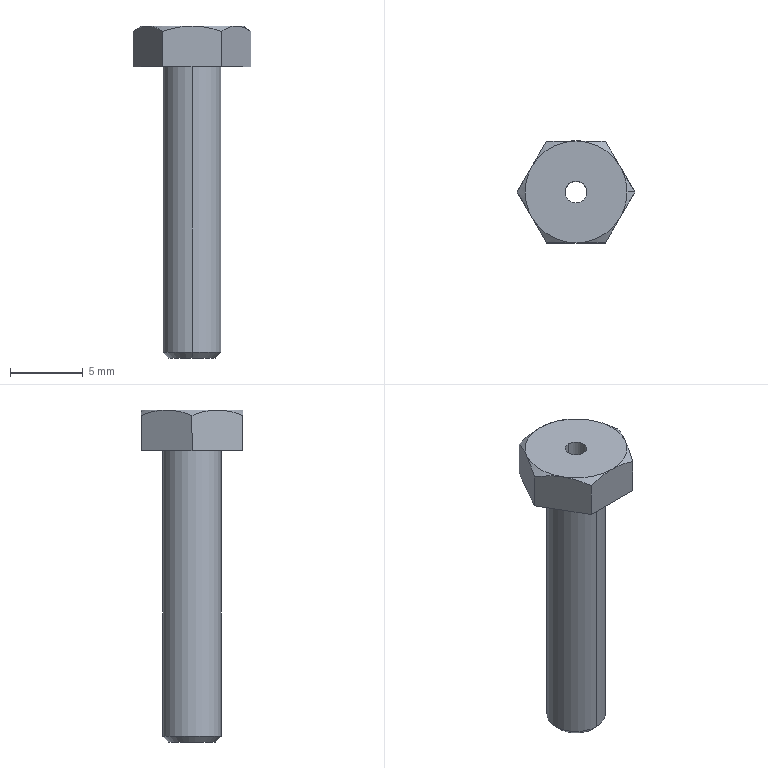Part | SolidWorks | features ICE 2, Chamfer 1, Revolution 1 | 1 solid | 22 faces | box 8.083 x 7 x 22.8 mm | volume 328.465 mm3 | cone 9 | plane 9 | cylinder 4 | commonest cylinder face diameters 1.5 x2 4 x2
STEP:
#1=CARTESIAN_POINT('',(0.,1.6,-20.));
#2=VERTEX_POINT('',#1);
#3=CARTESIAN_POINT('',(0.,-1.6,-20.));
#4=VERTEX_POINT('',#3);
#5=CARTESIAN_POINT('',(0.,0.,-20.));
#6=DIRECTION('',(0.,0.,-1.));
#7=DIRECTION('',(0.,-1.,0.));
#8=AXIS2_PLACEMENT_3D('',#5,#6,#7);
#9=CIRCLE('',#8,1.6);
#10=EDGE_CURVE('',#2,#4,#9,.T.);
#11=ORIENTED_EDGE('',*,*,#10,.F.);
#12=CARTESIAN_POINT('',(0.,2.,-19.6));
#13=VERTEX_POINT('',#12);
#14=CARTESIAN_POINT('',(0.,2.,-19.6));
#15=DIRECTION('',(0.,0.7071,0.7071));
#16=VECTOR('',#15,1000.);
#17=LINE('',#14,#16);
#18=EDGE_CURVE('',#2,#13,#17,.T.);
#19=ORIENTED_EDGE('',*,*,#18,.T.);
#20=CARTESIAN_POINT('',(0.,-2.,-19.6));
#21=VERTEX_POINT('',#20);
#22=CARTESIAN_POINT('',(0.,0.,-19.6));
#23=DIRECTION('',(0.,0.,1.));
#24=DIRECTION('',(0.,-1.,0.));
#25=AXIS2_PLACEMENT_3D('',#22,#23,#24);
#26=CIRCLE('',#25,2.);
#27=EDGE_CURVE('',#21,#13,#26,.T.);
#28=ORIENTED_EDGE('',*,*,#27,.F.);
#29=CARTESIAN_POINT('',(0.,-2.,-19.6));
#30=DIRECTION('',(0.,-0.7071,0.7071));
#31=VECTOR('',#30,1000.);
#32=LINE('',#29,#31);
#33=EDGE_CURVE('',#4,#21,#32,.T.);
#34=ORIENTED_EDGE('',*,*,#33,.F.);
#35=EDGE_LOOP('',(#11,#19,#28,#34));
#36=FACE_OUTER_BOUND('',#35,.T.);
#37=CARTESIAN_POINT('',(0.,0.,-19.6));
#38=DIRECTION('',(0.,0.,1.));
#39=DIRECTION('',(0.,-1.,0.));
#40=AXIS2_PLACEMENT_3D('',#37,#38,#39);
#41=CONICAL_SURFACE('',#40,2.,0.7854);
#42=ADVANCED_FACE('',(#36),#41,.T.);
#43=CARTESIAN_POINT('',(3.5,0.,2.8));
#44=VERTEX_POINT('',#43);
#45=CARTESIAN_POINT('',(3.031,1.75,2.8));
#46=VERTEX_POINT('',#45);
#47=CARTESIAN_POINT('',(0.,0.,2.8));
#48=DIRECTION('',(0.,0.,1.));
#49=DIRECTION('',(1.,0.,0.));
#50=AXIS2_PLACEMENT_3D('',#47,#48,#49);
#51=CIRCLE('',#50,3.5);
#52=EDGE_CURVE('',#44,#46,#51,.T.);
#53=ORIENTED_EDGE('',*,*,#52,.F.);
#54=CARTESIAN_POINT('',(4.041,0.,2.421));
#55=VERTEX_POINT('',#54);
#56=CARTESIAN_POINT('',(3.5,0.,2.8));
#57=DIRECTION('',(0.8192,0.,-0.5736));
#58=VECTOR('',#57,1000.);
#59=LINE('',#56,#58);
#60=EDGE_CURVE('',#44,#55,#59,.T.);
#61=ORIENTED_EDGE('',*,*,#60,.T.);
#62=CARTESIAN_POINT('',(3.031,1.75,2.8));
#63=CARTESIAN_POINT('',(3.117,1.601,2.8));
#64=CARTESIAN_POINT('',(3.204,1.45,2.791));
#65=CARTESIAN_POINT('',(3.376,1.153,2.756));
#66=CARTESIAN_POINT('',(3.461,1.006,2.73));
#67=CARTESIAN_POINT('',(3.713,0.569,2.63));
#68=CARTESIAN_POINT('',(3.878,0.2828,2.535));
#69=CARTESIAN_POINT('',(4.041,0.,2.421));
#70=B_SPLINE_CURVE_WITH_KNOTS('',3,(#62,#63,#64,#65,#66,#67,#68,#69),.UNSPECIFIED.,.F.,.F.,(4,2,2,4),(0.002056,0.002566,0.003076,0.004096),.UNSPECIFIED.);
#71=EDGE_CURVE('',#46,#55,#70,.T.);
#72=ORIENTED_EDGE('',*,*,#71,.F.);
#73=EDGE_LOOP('',(#53,#61,#72));
#74=FACE_OUTER_BOUND('',#73,.T.);
#75=CARTESIAN_POINT('',(0.,0.,2.8));
#76=DIRECTION('',(0.,0.,-1.));
#77=DIRECTION('',(1.,0.,0.));
#78=AXIS2_PLACEMENT_3D('',#75,#76,#77);
#79=CONICAL_SURFACE('',#78,3.5,0.9599);
#80=ADVANCED_FACE('',(#74),#79,.T.);
#81=CARTESIAN_POINT('',(0.,0.75,-20.));
#82=VERTEX_POINT('',#81);
#83=CARTESIAN_POINT('',(0.,-0.75,-20.));
#84=VERTEX_POINT('',#83);
#85=CARTESIAN_POINT('',(0.,0.,-20.));
#86=DIRECTION('',(0.,0.,1.));
#87=DIRECTION('',(0.,-1.,0.));
#88=AXIS2_PLACEMENT_3D('',#85,#86,#87);
#89=CIRCLE('',#88,0.75);
#90=EDGE_CURVE('',#82,#84,#89,.T.);
#91=ORIENTED_EDGE('',*,*,#90,.F.);
#92=CARTESIAN_POINT('',(0.,0.75,2.8));
#93=VERTEX_POINT('',#92);
#94=CARTESIAN_POINT('',(0.,0.75,2.8));
#95=DIRECTION('',(0.,0.,1.));
#96=VECTOR('',#95,1000.);
#97=LINE('',#94,#96);
#98=EDGE_CURVE('',#82,#93,#97,.T.);
#99=ORIENTED_EDGE('',*,*,#98,.T.);
#100=CARTESIAN_POINT('',(0.,-0.75,2.8));
#101=VERTEX_POINT('',#100);
#102=CARTESIAN_POINT('',(0.,0.,2.8));
#103=DIRECTION('',(0.,0.,1.));
#104=DIRECTION('',(0.,-1.,0.));
#105=AXIS2_PLACEMENT_3D('',#102,#103,#104);
#106=CIRCLE('',#105,0.75);
#107=EDGE_CURVE('',#93,#101,#106,.T.);
#108=ORIENTED_EDGE('',*,*,#107,.T.);
#109=CARTESIAN_POINT('',(0.,-0.75,2.8));
#110=DIRECTION('',(0.,0.,1.));
#111=VECTOR('',#110,1000.);
#112=LINE('',#109,#111);
#113=EDGE_CURVE('',#84,#101,#112,.T.);
#114=ORIENTED_EDGE('',*,*,#113,.F.);
#115=EDGE_LOOP('',(#91,#99,#108,#114));
#116=FACE_OUTER_BOUND('',#115,.T.);
#117=CARTESIAN_POINT('',(0.,0.,2.8));
#118=DIRECTION('',(0.,0.,1.));
#119=DIRECTION('',(0.,-1.,0.));
#120=AXIS2_PLACEMENT_3D('',#117,#118,#119);
#121=CYLINDRICAL_SURFACE('',#120,0.75);
#122=ADVANCED_FACE('',(#116),#121,.F.);
#123=ORIENTED_EDGE('',*,*,#27,.T.);
#124=CARTESIAN_POINT('',(0.,2.,0.));
#125=VERTEX_POINT('',#124);
#126=CARTESIAN_POINT('',(0.,2.,2.8));
#127=DIRECTION('',(0.,0.,1.));
#128=VECTOR('',#127,1000.);
#129=LINE('',#126,#128);
#130=EDGE_CURVE('',#13,#125,#129,.T.);
#131=ORIENTED_EDGE('',*,*,#130,.T.);
#132=CARTESIAN_POINT('',(0.,-2.,0.));
#133=VERTEX_POINT('',#132);
#134=CARTESIAN_POINT('',(0.,0.,0.));
#135=DIRECTION('',(0.,0.,1.));
#136=DIRECTION('',(1.,0.,0.));
#137=AXIS2_PLACEMENT_3D('',#134,#135,#136);
#138=CIRCLE('',#137,2.);
#139=EDGE_CURVE('',#133,#125,#138,.T.);
#140=ORIENTED_EDGE('',*,*,#139,.F.);
#141=CARTESIAN_POINT('',(0.,-2.,2.8));
#142=DIRECTION('',(0.,0.,1.));
#143=VECTOR('',#142,1000.);
#144=LINE('',#141,#143);
#145=EDGE_CURVE('',#21,#133,#144,.T.);
#146=ORIENTED_EDGE('',*,*,#145,.F.);
#147=EDGE_LOOP('',(#123,#131,#140,#146));
#148=FACE_OUTER_BOUND('',#147,.T.);
#149=CARTESIAN_POINT('',(0.,0.,2.8));
#150=DIRECTION('',(0.,0.,1.));
#151=DIRECTION('',(0.,-1.,0.));
#152=AXIS2_PLACEMENT_3D('',#149,#150,#151);
#153=CYLINDRICAL_SURFACE('',#152,2.);
#154=ADVANCED_FACE('',(#148),#153,.T.);
#155=CARTESIAN_POINT('',(0.,0.,2.8));
#156=DIRECTION('',(0.,0.,1.));
#157=DIRECTION('',(0.,-1.,0.));
#158=AXIS2_PLACEMENT_3D('',#155,#156,#157);
#159=CIRCLE('',#158,0.75);
#160=EDGE_CURVE('',#101,#93,#159,.T.);
#161=ORIENTED_EDGE('',*,*,#160,.F.);
#162=ORIENTED_EDGE('',*,*,#107,.F.);
#163=EDGE_LOOP('',(#161,#162));
#164=FACE_BOUND('',#163,.T.);
#165=CARTESIAN_POINT('',(0.,3.5,2.8));
#166=VERTEX_POINT('',#165);
#167=CARTESIAN_POINT('',(0.,0.,2.8));
#168=DIRECTION('',(0.,0.,1.));
#169=DIRECTION('',(1.,0.,0.));
#170=AXIS2_PLACEMENT_3D('',#167,#168,#169);
#171=CIRCLE('',#170,3.5);
#172=EDGE_CURVE('',#46,#166,#171,.T.);
#173=ORIENTED_EDGE('',*,*,#172,.T.);
#174=CARTESIAN_POINT('',(-3.031,1.75,2.8));
#175=VERTEX_POINT('',#174);
#176=CARTESIAN_POINT('',(0.,0.,2.8));
#177=DIRECTION('',(0.,0.,1.));
#178=DIRECTION('',(1.,0.,0.));
#179=AXIS2_PLACEMENT_3D('',#176,#177,#178);
#180=CIRCLE('',#179,3.5);
#181=EDGE_CURVE('',#166,#175,#180,.T.);
#182=ORIENTED_EDGE('',*,*,#181,.T.);
#183=CARTESIAN_POINT('',(-3.031,-1.75,2.8));
#184=VERTEX_POINT('',#183);
#185=CARTESIAN_POINT('',(0.,0.,2.8));
#186=DIRECTION('',(0.,0.,1.));
#187=DIRECTION('',(1.,0.,0.));
#188=AXIS2_PLACEMENT_3D('',#185,#186,#187);
#189=CIRCLE('',#188,3.5);
#190=EDGE_CURVE('',#175,#184,#189,.T.);
#191=ORIENTED_EDGE('',*,*,#190,.T.);
#192=CARTESIAN_POINT('',(0.,-3.5,2.8));
#193=VERTEX_POINT('',#192);
#194=CARTESIAN_POINT('',(0.,0.,2.8));
#195=DIRECTION('',(0.,0.,1.));
#196=DIRECTION('',(1.,0.,0.));
#197=AXIS2_PLACEMENT_3D('',#194,#195,#196);
#198=CIRCLE('',#197,3.5);
#199=EDGE_CURVE('',#184,#193,#198,.T.);
#200=ORIENTED_EDGE('',*,*,#199,.T.);
#201=CARTESIAN_POINT('',(3.031,-1.75,2.8));
#202=VERTEX_POINT('',#201);
#203=CARTESIAN_POINT('',(0.,0.,2.8));
#204=DIRECTION('',(0.,0.,1.));
#205=DIRECTION('',(1.,0.,0.));
#206=AXIS2_PLACEMENT_3D('',#203,#204,#205);
#207=CIRCLE('',#206,3.5);
#208=EDGE_CURVE('',#193,#202,#207,.T.);
#209=ORIENTED_EDGE('',*,*,#208,.T.);
#210=CARTESIAN_POINT('',(0.,0.,2.8));
#211=DIRECTION('',(0.,0.,1.));
#212=DIRECTION('',(1.,0.,0.));
#213=AXIS2_PLACEMENT_3D('',#210,#211,#212);
#214=CIRCLE('',#213,3.5);
#215=EDGE_CURVE('',#202,#44,#214,.T.);
#216=ORIENTED_EDGE('',*,*,#215,.T.);
#217=ORIENTED_EDGE('',*,*,#52,.T.);
#218=EDGE_LOOP('',(#173,#182,#191,#200,#209,#216,#217));
#219=FACE_OUTER_BOUND('',#218,.T.);
#220=CARTESIAN_POINT('',(0.,2.,2.8));
#221=DIRECTION('',(0.,0.,-1.));
#222=DIRECTION('',(0.,1.,0.));
#223=AXIS2_PLACEMENT_3D('',#220,#221,#222);
#224=PLANE('',#223);
#225=ADVANCED_FACE('',(#164,#219),#224,.F.);
#226=CARTESIAN_POINT('',(2.021,3.5,0.));
#227=VERTEX_POINT('',#226);
#228=CARTESIAN_POINT('',(2.021,3.5,2.421));
#229=VERTEX_POINT('',#228);
#230=CARTESIAN_POINT('',(2.021,3.5,0.));
#231=DIRECTION('',(0.,0.,1.));
#232=VECTOR('',#231,1000.);
#233=LINE('',#230,#232);
#234=EDGE_CURVE('',#227,#229,#233,.T.);
#235=ORIENTED_EDGE('',*,*,#234,.T.);
#236=CARTESIAN_POINT('',(2.021,3.5,2.421));
#237=CARTESIAN_POINT('',(2.349,2.932,2.651));
#238=CARTESIAN_POINT('',(2.684,2.352,2.8));
#239=CARTESIAN_POINT('',(3.031,1.75,2.8));
#240=B_SPLINE_CURVE_WITH_KNOTS('',3,(#236,#237,#238,#239),.UNSPECIFIED.,.F.,.F.,(4,4),(0.000000241,0.002056),.UNSPECIFIED.);
#241=EDGE_CURVE('',#229,#46,#240,.T.);
#242=ORIENTED_EDGE('',*,*,#241,.T.);
#243=ORIENTED_EDGE('',*,*,#71,.T.);
#244=CARTESIAN_POINT('',(4.041,0.,0.));
#245=VERTEX_POINT('',#244);
#246=CARTESIAN_POINT('',(4.041,0.,0.));
#247=DIRECTION('',(0.,0.,1.));
#248=VECTOR('',#247,1000.);
#249=LINE('',#246,#248);
#250=EDGE_CURVE('',#245,#55,#249,.T.);
#251=ORIENTED_EDGE('',*,*,#250,.F.);
#252=CARTESIAN_POINT('',(4.041,0.,0.));
#253=DIRECTION('',(-0.5,0.866,0.));
#254=VECTOR('',#253,1000.);
#255=LINE('',#252,#254);
#256=EDGE_CURVE('',#245,#227,#255,.T.);
#257=ORIENTED_EDGE('',*,*,#256,.T.);
#258=EDGE_LOOP('',(#235,#242,#243,#251,#257));
#259=FACE_OUTER_BOUND('',#258,.T.);
#260=CARTESIAN_POINT('',(4.041,0.,0.));
#261=DIRECTION('',(0.866,0.5,0.));
#262=DIRECTION('',(-0.5,0.866,0.));
#263=AXIS2_PLACEMENT_3D('',#260,#261,#262);
#264=PLANE('',#263);
#265=ADVANCED_FACE('',(#259),#264,.T.);
#266=ORIENTED_EDGE('',*,*,#250,.T.);
#267=CARTESIAN_POINT('',(4.041,0.,2.421));
#268=CARTESIAN_POINT('',(3.713,-0.5682,2.651));
#269=CARTESIAN_POINT('',(3.379,-1.148,2.8));
#270=CARTESIAN_POINT('',(3.031,-1.75,2.8));
#271=B_SPLINE_CURVE_WITH_KNOTS('',3,(#267,#268,#269,#270),.UNSPECIFIED.,.F.,.F.,(4,4),(0.000000241,0.002056),.UNSPECIFIED.);
#272=EDGE_CURVE('',#55,#202,#271,.T.);
#273=ORIENTED_EDGE('',*,*,#272,.T.);
#274=CARTESIAN_POINT('',(2.021,-3.5,2.421));
#275=VERTEX_POINT('',#274);
#276=CARTESIAN_POINT('',(3.031,-1.75,2.8));
#277=CARTESIAN_POINT('',(2.945,-1.899,2.8));
#278=CARTESIAN_POINT('',(2.858,-2.05,2.791));
#279=CARTESIAN_POINT('',(2.686,-2.347,2.756));
#280=CARTESIAN_POINT('',(2.602,-2.494,2.73));
#281=CARTESIAN_POINT('',(2.349,-2.931,2.63));
#282=CARTESIAN_POINT('',(2.184,-3.217,2.535));
#283=CARTESIAN_POINT('',(2.021,-3.5,2.421));
#284=B_SPLINE_CURVE_WITH_KNOTS('',3,(#276,#277,#278,#279,#280,#281,#282,#283),.UNSPECIFIED.,.F.,.F.,(4,2,2,4),(0.002056,0.002566,0.003076,0.004096),.UNSPECIFIED.);
#285=EDGE_CURVE('',#202,#275,#284,.T.);
#286=ORIENTED_EDGE('',*,*,#285,.T.);
#287=CARTESIAN_POINT('',(2.021,-3.5,0.));
#288=VERTEX_POINT('',#287);
#289=CARTESIAN_POINT('',(2.021,-3.5,0.));
#290=DIRECTION('',(0.,0.,1.));
#291=VECTOR('',#290,1000.);
#292=LINE('',#289,#291);
#293=EDGE_CURVE('',#288,#275,#292,.T.);
#294=ORIENTED_EDGE('',*,*,#293,.F.);
#295=CARTESIAN_POINT('',(2.021,-3.5,0.));
#296=DIRECTION('',(0.5,0.866,0.));
#297=VECTOR('',#296,1000.);
#298=LINE('',#295,#297);
#299=EDGE_CURVE('',#288,#245,#298,.T.);
#300=ORIENTED_EDGE('',*,*,#299,.T.);
#301=EDGE_LOOP('',(#266,#273,#286,#294,#300));
#302=FACE_OUTER_BOUND('',#301,.T.);
#303=CARTESIAN_POINT('',(2.021,-3.5,0.));
#304=DIRECTION('',(0.866,-0.5,0.));
#305=DIRECTION('',(0.5,0.866,0.));
#306=AXIS2_PLACEMENT_3D('',#303,#304,#305);
#307=PLANE('',#306);
#308=ADVANCED_FACE('',(#302),#307,.T.);
#309=ORIENTED_EDGE('',*,*,#293,.T.);
#310=CARTESIAN_POINT('',(2.021,-3.5,2.421));
#311=CARTESIAN_POINT('',(1.697,-3.5,2.534));
#312=CARTESIAN_POINT('',(1.367,-3.5,2.629));
#313=CARTESIAN_POINT('',(0.6927,-3.5,2.763));
#314=CARTESIAN_POINT('',(0.3434,-3.5,2.8));
#315=CARTESIAN_POINT('',(0.,-3.5,2.8));
#316=B_SPLINE_CURVE_WITH_KNOTS('',3,(#310,#311,#312,#313,#314,#315),.UNSPECIFIED.,.F.,.F.,(4,2,4),(0.008163,0.009192,0.01022),.UNSPECIFIED.);
#317=EDGE_CURVE('',#275,#193,#316,.T.);
#318=ORIENTED_EDGE('',*,*,#317,.T.);
#319=CARTESIAN_POINT('',(-2.021,-3.5,2.421));
#320=VERTEX_POINT('',#319);
#321=CARTESIAN_POINT('',(0.,-3.5,2.8));
#322=CARTESIAN_POINT('',(-0.344,-3.5,2.8));
#323=CARTESIAN_POINT('',(-0.6844,-3.5,2.764));
#324=CARTESIAN_POINT('',(-1.359,-3.5,2.631));
#325=CARTESIAN_POINT('',(-1.695,-3.5,2.535));
#326=CARTESIAN_POINT('',(-2.021,-3.5,2.421));
#327=B_SPLINE_CURVE_WITH_KNOTS('',3,(#321,#322,#323,#324,#325,#326),.UNSPECIFIED.,.F.,.F.,(4,2,4),(0.01022,0.01125,0.01228),.UNSPECIFIED.);
#328=EDGE_CURVE('',#193,#320,#327,.T.);
#329=ORIENTED_EDGE('',*,*,#328,.T.);
#330=CARTESIAN_POINT('',(-2.021,-3.5,0.));
#331=VERTEX_POINT('',#330);
#332=CARTESIAN_POINT('',(-2.021,-3.5,0.));
#333=DIRECTION('',(0.,0.,1.));
#334=VECTOR('',#333,1000.);
#335=LINE('',#332,#334);
#336=EDGE_CURVE('',#331,#320,#335,.T.);
#337=ORIENTED_EDGE('',*,*,#336,.F.);
#338=CARTESIAN_POINT('',(-2.021,-3.5,0.));
#339=DIRECTION('',(1.,0.,0.));
#340=VECTOR('',#339,1000.);
#341=LINE('',#338,#340);
#342=EDGE_CURVE('',#331,#288,#341,.T.);
#343=ORIENTED_EDGE('',*,*,#342,.T.);
#344=EDGE_LOOP('',(#309,#318,#329,#337,#343));
#345=FACE_OUTER_BOUND('',#344,.T.);
#346=CARTESIAN_POINT('',(-2.021,-3.5,0.));
#347=DIRECTION('',(0.,-1.,0.));
#348=DIRECTION('',(1.,0.,0.));
#349=AXIS2_PLACEMENT_3D('',#346,#347,#348);
#350=PLANE('',#349);
#351=ADVANCED_FACE('',(#345),#350,.T.);
#352=ORIENTED_EDGE('',*,*,#336,.T.);
#353=CARTESIAN_POINT('',(-2.021,-3.5,2.421));
#354=CARTESIAN_POINT('',(-2.349,-2.932,2.651));
#355=CARTESIAN_POINT('',(-2.684,-2.352,2.8));
#356=CARTESIAN_POINT('',(-3.031,-1.75,2.8));
#357=B_SPLINE_CURVE_WITH_KNOTS('',3,(#353,#354,#355,#356),.UNSPECIFIED.,.F.,.F.,(4,4),(0.000000241,0.002056),.UNSPECIFIED.);
#358=EDGE_CURVE('',#320,#184,#357,.T.);
#359=ORIENTED_EDGE('',*,*,#358,.T.);
#360=CARTESIAN_POINT('',(-4.041,0.,2.421));
#361=VERTEX_POINT('',#360);
#362=CARTESIAN_POINT('',(-3.031,-1.75,2.8));
#363=CARTESIAN_POINT('',(-3.117,-1.601,2.8));
#364=CARTESIAN_POINT('',(-3.204,-1.45,2.791));
#365=CARTESIAN_POINT('',(-3.376,-1.153,2.756));
#366=CARTESIAN_POINT('',(-3.461,-1.006,2.73));
#367=CARTESIAN_POINT('',(-3.713,-0.569,2.63));
#368=CARTESIAN_POINT('',(-3.878,-0.2828,2.535));
#369=CARTESIAN_POINT('',(-4.041,0.,2.421));
#370=B_SPLINE_CURVE_WITH_KNOTS('',3,(#362,#363,#364,#365,#366,#367,#368,#369),.UNSPECIFIED.,.F.,.F.,(4,2,2,4),(0.002056,0.002566,0.003076,0.004096),.UNSPECIFIED.);
#371=EDGE_CURVE('',#184,#361,#370,.T.);
#372=ORIENTED_EDGE('',*,*,#371,.T.);
#373=CARTESIAN_POINT('',(-4.041,0.,0.));
#374=VERTEX_POINT('',#373);
#375=CARTESIAN_POINT('',(-4.041,0.,0.));
#376=DIRECTION('',(0.,0.,1.));
#377=VECTOR('',#376,1000.);
#378=LINE('',#375,#377);
#379=EDGE_CURVE('',#374,#361,#378,.T.);
#380=ORIENTED_EDGE('',*,*,#379,.F.);
#381=CARTESIAN_POINT('',(-4.041,0.,0.));
#382=DIRECTION('',(0.5,-0.866,0.));
#383=VECTOR('',#382,1000.);
#384=LINE('',#381,#383);
#385=EDGE_CURVE('',#374,#331,#384,.T.);
#386=ORIENTED_EDGE('',*,*,#385,.T.);
#387=EDGE_LOOP('',(#352,#359,#372,#380,#386));
#388=FACE_OUTER_BOUND('',#387,.T.);
#389=CARTESIAN_POINT('',(-4.041,0.,0.));
#390=DIRECTION('',(-0.866,-0.5,0.));
#391=DIRECTION('',(0.5,-0.866,0.));
#392=AXIS2_PLACEMENT_3D('',#389,#390,#391);
#393=PLANE('',#392);
#394=ADVANCED_FACE('',(#388),#393,.T.);
#395=ORIENTED_EDGE('',*,*,#379,.T.);
#396=CARTESIAN_POINT('',(-4.041,0.,2.421));
#397=CARTESIAN_POINT('',(-3.713,0.5682,2.651));
#398=CARTESIAN_POINT('',(-3.379,1.148,2.8));
#399=CARTESIAN_POINT('',(-3.031,1.75,2.8));
#400=B_SPLINE_CURVE_WITH_KNOTS('',3,(#396,#397,#398,#399),.UNSPECIFIED.,.F.,.F.,(4,4),(0.000000241,0.002056),.UNSPECIFIED.);
#401=EDGE_CURVE('',#361,#175,#400,.T.);
#402=ORIENTED_EDGE('',*,*,#401,.T.);
#403=CARTESIAN_POINT('',(-2.021,3.5,2.421));
#404=VERTEX_POINT('',#403);
#405=CARTESIAN_POINT('',(-3.031,1.75,2.8));
#406=CARTESIAN_POINT('',(-2.945,1.899,2.8));
#407=CARTESIAN_POINT('',(-2.858,2.05,2.791));
#408=CARTESIAN_POINT('',(-2.686,2.347,2.756));
#409=CARTESIAN_POINT('',(-2.602,2.494,2.73));
#410=CARTESIAN_POINT('',(-2.349,2.931,2.63));
#411=CARTESIAN_POINT('',(-2.184,3.217,2.535));
#412=CARTESIAN_POINT('',(-2.021,3.5,2.421));
#413=B_SPLINE_CURVE_WITH_KNOTS('',3,(#405,#406,#407,#408,#409,#410,#411,#412),.UNSPECIFIED.,.F.,.F.,(4,2,2,4),(0.002056,0.002566,0.003076,0.004096),.UNSPECIFIED.);
#414=EDGE_CURVE('',#175,#404,#413,.T.);
#415=ORIENTED_EDGE('',*,*,#414,.T.);
#416=CARTESIAN_POINT('',(-2.021,3.5,0.));
#417=VERTEX_POINT('',#416);
#418=CARTESIAN_POINT('',(-2.021,3.5,0.));
#419=DIRECTION('',(0.,0.,1.));
#420=VECTOR('',#419,1000.);
#421=LINE('',#418,#420);
#422=EDGE_CURVE('',#417,#404,#421,.T.);
#423=ORIENTED_EDGE('',*,*,#422,.F.);
#424=CARTESIAN_POINT('',(-2.021,3.5,0.));
#425=DIRECTION('',(-0.5,-0.866,0.));
#426=VECTOR('',#425,1000.);
#427=LINE('',#424,#426);
#428=EDGE_CURVE('',#417,#374,#427,.T.);
#429=ORIENTED_EDGE('',*,*,#428,.T.);
#430=EDGE_LOOP('',(#395,#402,#415,#423,#429));
#431=FACE_OUTER_BOUND('',#430,.T.);
#432=CARTESIAN_POINT('',(-2.021,3.5,0.));
#433=DIRECTION('',(-0.866,0.5,0.));
#434=DIRECTION('',(-0.5,-0.866,0.));
#435=AXIS2_PLACEMENT_3D('',#432,#433,#434);
#436=PLANE('',#435);
#437=ADVANCED_FACE('',(#431),#436,.T.);
#438=ORIENTED_EDGE('',*,*,#422,.T.);
#439=CARTESIAN_POINT('',(-2.021,3.5,2.421));
#440=CARTESIAN_POINT('',(-1.695,3.5,2.535));
#441=CARTESIAN_POINT('',(-1.359,3.5,2.631));
#442=CARTESIAN_POINT('',(-0.6844,3.5,2.764));
#443=CARTESIAN_POINT('',(-0.344,3.5,2.8));
#444=CARTESIAN_POINT('',(0.,3.5,2.8));
#445=B_SPLINE_CURVE_WITH_KNOTS('',3,(#439,#440,#441,#442,#443,#444),.UNSPECIFIED.,.F.,.F.,(4,2,4),(0.003234,0.004263,0.005293),.UNSPECIFIED.);
#446=EDGE_CURVE('',#404,#166,#445,.T.);
#447=ORIENTED_EDGE('',*,*,#446,.T.);
#448=CARTESIAN_POINT('',(0.,3.5,2.8));
#449=CARTESIAN_POINT('',(0.3434,3.5,2.8));
#450=CARTESIAN_POINT('',(0.6927,3.5,2.763));
#451=CARTESIAN_POINT('',(1.367,3.5,2.629));
#452=CARTESIAN_POINT('',(1.697,3.5,2.534));
#453=CARTESIAN_POINT('',(2.021,3.5,2.421));
#454=B_SPLINE_CURVE_WITH_KNOTS('',3,(#448,#449,#450,#451,#452,#453),.UNSPECIFIED.,.F.,.F.,(4,2,4),(0.005293,0.006321,0.007348),.UNSPECIFIED.);
#455=EDGE_CURVE('',#166,#229,#454,.T.);
#456=ORIENTED_EDGE('',*,*,#455,.T.);
#457=ORIENTED_EDGE('',*,*,#234,.F.);
#458=CARTESIAN_POINT('',(2.021,3.5,0.));
#459=DIRECTION('',(-1.,0.,0.));
#460=VECTOR('',#459,1000.);
#461=LINE('',#458,#460);
#462=EDGE_CURVE('',#227,#417,#461,.T.);
#463=ORIENTED_EDGE('',*,*,#462,.T.);
#464=EDGE_LOOP('',(#438,#447,#456,#457,#463));
#465=FACE_OUTER_BOUND('',#464,.T.);
#466=CARTESIAN_POINT('',(2.021,3.5,0.));
#467=DIRECTION('',(0.,1.,0.));
#468=DIRECTION('',(-1.,0.,0.));
#469=AXIS2_PLACEMENT_3D('',#466,#467,#468);
#470=PLANE('',#469);
#471=ADVANCED_FACE('',(#465),#470,.T.);
#472=ORIENTED_EDGE('',*,*,#130,.F.);
#473=CARTESIAN_POINT('',(0.,0.,-19.6));
#474=DIRECTION('',(0.,0.,1.));
#475=DIRECTION('',(0.,-1.,0.));
#476=AXIS2_PLACEMENT_3D('',#473,#474,#475);
#477=CIRCLE('',#476,2.);
#478=EDGE_CURVE('',#13,#21,#477,.T.);
#479=ORIENTED_EDGE('',*,*,#478,.T.);
#480=ORIENTED_EDGE('',*,*,#145,.T.);
#481=CARTESIAN_POINT('',(0.,0.,0.));
#482=DIRECTION('',(0.,0.,1.));
#483=DIRECTION('',(1.,0.,0.));
#484=AXIS2_PLACEMENT_3D('',#481,#482,#483);
#485=CIRCLE('',#484,2.);
#486=EDGE_CURVE('',#125,#133,#485,.T.);
#487=ORIENTED_EDGE('',*,*,#486,.F.);
#488=EDGE_LOOP('',(#472,#479,#480,#487));
#489=FACE_OUTER_BOUND('',#488,.T.);
#490=CARTESIAN_POINT('',(0.,0.,2.8));
#491=DIRECTION('',(0.,0.,1.));
#492=DIRECTION('',(0.,-1.,0.));
#493=AXIS2_PLACEMENT_3D('',#490,#491,#492);
#494=CYLINDRICAL_SURFACE('',#493,2.);
#495=ADVANCED_FACE('',(#489),#494,.T.);
#496=CARTESIAN_POINT('',(0.,0.,-20.));
#497=DIRECTION('',(0.,0.,-1.));
#498=DIRECTION('',(0.,-1.,0.));
#499=AXIS2_PLACEMENT_3D('',#496,#497,#498);
#500=CIRCLE('',#499,1.6);
#501=EDGE_CURVE('',#4,#2,#500,.T.);
#502=ORIENTED_EDGE('',*,*,#501,.T.);
#503=ORIENTED_EDGE('',*,*,#10,.T.);
#504=EDGE_LOOP('',(#502,#503));
#505=FACE_OUTER_BOUND('',#504,.T.);
#506=CARTESIAN_POINT('',(0.,0.,-20.));
#507=DIRECTION('',(0.,0.,1.));
#508=DIRECTION('',(0.,-1.,0.));
#509=AXIS2_PLACEMENT_3D('',#506,#507,#508);
#510=CIRCLE('',#509,0.75);
#511=EDGE_CURVE('',#84,#82,#510,.T.);
#512=ORIENTED_EDGE('',*,*,#511,.T.);
#513=ORIENTED_EDGE('',*,*,#90,.T.);
#514=EDGE_LOOP('',(#512,#513));
#515=FACE_BOUND('',#514,.T.);
#516=CARTESIAN_POINT('',(0.,2.,-20.));
#517=DIRECTION('',(0.,0.,1.));
#518=DIRECTION('',(0.,-1.,0.));
#519=AXIS2_PLACEMENT_3D('',#516,#517,#518);
#520=PLANE('',#519);
#521=ADVANCED_FACE('',(#505,#515),#520,.F.);
#522=ORIENTED_EDGE('',*,*,#98,.F.);
#523=ORIENTED_EDGE('',*,*,#511,.F.);
#524=ORIENTED_EDGE('',*,*,#113,.T.);
#525=ORIENTED_EDGE('',*,*,#160,.T.);
#526=EDGE_LOOP('',(#522,#523,#524,#525));
#527=FACE_OUTER_BOUND('',#526,.T.);
#528=CARTESIAN_POINT('',(0.,0.,2.8));
#529=DIRECTION('',(0.,0.,1.));
#530=DIRECTION('',(0.,-1.,0.));
#531=AXIS2_PLACEMENT_3D('',#528,#529,#530);
#532=CYLINDRICAL_SURFACE('',#531,0.75);
#533=ADVANCED_FACE('',(#527),#532,.F.);
#534=ORIENTED_EDGE('',*,*,#256,.F.);
#535=ORIENTED_EDGE('',*,*,#299,.F.);
#536=ORIENTED_EDGE('',*,*,#342,.F.);
#537=ORIENTED_EDGE('',*,*,#385,.F.);
#538=ORIENTED_EDGE('',*,*,#428,.F.);
#539=ORIENTED_EDGE('',*,*,#462,.F.);
#540=EDGE_LOOP('',(#534,#535,#536,#537,#538,#539));
#541=FACE_OUTER_BOUND('',#540,.T.);
#542=ORIENTED_EDGE('',*,*,#139,.T.);
#543=ORIENTED_EDGE('',*,*,#486,.T.);
#544=EDGE_LOOP('',(#542,#543));
#545=FACE_BOUND('',#544,.T.);
#546=CARTESIAN_POINT('',(2.021,3.5,0.));
#547=DIRECTION('',(0.,0.,1.));
#548=DIRECTION('',(1.,0.,0.));
#549=AXIS2_PLACEMENT_3D('',#546,#547,#548);
#550=PLANE('',#549);
#551=ADVANCED_FACE('',(#541,#545),#550,.F.);
#552=ORIENTED_EDGE('',*,*,#455,.F.);
#553=ORIENTED_EDGE('',*,*,#172,.F.);
#554=ORIENTED_EDGE('',*,*,#241,.F.);
#555=EDGE_LOOP('',(#552,#553,#554));
#556=FACE_OUTER_BOUND('',#555,.T.);
#557=CARTESIAN_POINT('',(0.,0.,2.8));
#558=DIRECTION('',(0.,0.,-1.));
#559=DIRECTION('',(1.,0.,0.));
#560=AXIS2_PLACEMENT_3D('',#557,#558,#559);
#561=CONICAL_SURFACE('',#560,3.5,0.9599);
#562=ADVANCED_FACE('',(#556),#561,.T.);
#563=ORIENTED_EDGE('',*,*,#181,.F.);
#564=ORIENTED_EDGE('',*,*,#446,.F.);
#565=ORIENTED_EDGE('',*,*,#414,.F.);
#566=EDGE_LOOP('',(#563,#564,#565));
#567=FACE_OUTER_BOUND('',#566,.T.);
#568=CARTESIAN_POINT('',(0.,0.,2.8));
#569=DIRECTION('',(0.,0.,-1.));
#570=DIRECTION('',(1.,0.,0.));
#571=AXIS2_PLACEMENT_3D('',#568,#569,#570);
#572=CONICAL_SURFACE('',#571,3.5,0.9599);
#573=ADVANCED_FACE('',(#567),#572,.T.);
#574=ORIENTED_EDGE('',*,*,#190,.F.);
#575=ORIENTED_EDGE('',*,*,#401,.F.);
#576=ORIENTED_EDGE('',*,*,#371,.F.);
#577=EDGE_LOOP('',(#574,#575,#576));
#578=FACE_OUTER_BOUND('',#577,.T.);
#579=CARTESIAN_POINT('',(0.,0.,2.8));
#580=DIRECTION('',(0.,0.,-1.));
#581=DIRECTION('',(1.,0.,0.));
#582=AXIS2_PLACEMENT_3D('',#579,#580,#581);
#583=CONICAL_SURFACE('',#582,3.5,0.9599);
#584=ADVANCED_FACE('',(#578),#583,.T.);
#585=ORIENTED_EDGE('',*,*,#199,.F.);
#586=ORIENTED_EDGE('',*,*,#358,.F.);
#587=ORIENTED_EDGE('',*,*,#328,.F.);
#588=EDGE_LOOP('',(#585,#586,#587));
#589=FACE_OUTER_BOUND('',#588,.T.);
#590=CARTESIAN_POINT('',(0.,0.,2.8));
#591=DIRECTION('',(0.,0.,-1.));
#592=DIRECTION('',(1.,0.,0.));
#593=AXIS2_PLACEMENT_3D('',#590,#591,#592);
#594=CONICAL_SURFACE('',#593,3.5,0.9599);
#595=ADVANCED_FACE('',(#589),#594,.T.);
#596=ORIENTED_EDGE('',*,*,#208,.F.);
#597=ORIENTED_EDGE('',*,*,#317,.F.);
#598=ORIENTED_EDGE('',*,*,#285,.F.);
#599=EDGE_LOOP('',(#596,#597,#598));
#600=FACE_OUTER_BOUND('',#599,.T.);
#601=CARTESIAN_POINT('',(0.,0.,2.8));
#602=DIRECTION('',(0.,0.,-1.));
#603=DIRECTION('',(1.,0.,0.));
#604=AXIS2_PLACEMENT_3D('',#601,#602,#603);
#605=CONICAL_SURFACE('',#604,3.5,0.9599);
#606=ADVANCED_FACE('',(#600),#605,.T.);
#607=ORIENTED_EDGE('',*,*,#60,.F.);
#608=ORIENTED_EDGE('',*,*,#215,.F.);
#609=ORIENTED_EDGE('',*,*,#272,.F.);
#610=EDGE_LOOP('',(#607,#608,#609));
#611=FACE_OUTER_BOUND('',#610,.T.);
#612=CARTESIAN_POINT('',(0.,0.,2.8));
#613=DIRECTION('',(0.,0.,-1.));
#614=DIRECTION('',(1.,0.,0.));
#615=AXIS2_PLACEMENT_3D('',#612,#613,#614);
#616=CONICAL_SURFACE('',#615,3.5,0.9599);
#617=ADVANCED_FACE('',(#611),#616,.T.);
#618=ORIENTED_EDGE('',*,*,#18,.F.);
#619=ORIENTED_EDGE('',*,*,#501,.F.);
#620=ORIENTED_EDGE('',*,*,#33,.T.);
#621=ORIENTED_EDGE('',*,*,#478,.F.);
#622=EDGE_LOOP('',(#618,#619,#620,#621));
#623=FACE_OUTER_BOUND('',#622,.T.);
#624=CARTESIAN_POINT('',(0.,0.,-19.6));
#625=DIRECTION('',(0.,0.,1.));
#626=DIRECTION('',(0.,-1.,0.));
#627=AXIS2_PLACEMENT_3D('',#624,#625,#626);
#628=CONICAL_SURFACE('',#627,2.,0.7854);
#629=ADVANCED_FACE('',(#623),#628,.T.);
#630=CLOSED_SHELL('',(#42,#80,#122,#154,#225,#265,#308,#351,#394,#437,#471,#495,#521,#533,#551,#562,#573,#584,#595,#606,#617,#629));
#631=MANIFOLD_SOLID_BREP('',#630);
#632=CARTESIAN_POINT('',(0.,0.,0.));
#633=DIRECTION('',(0.,0.,1.));
#634=DIRECTION('',(1.,0.,0.));
#635=AXIS2_PLACEMENT_3D('',#632,#633,#634);
#636=(LENGTH_UNIT()NAMED_UNIT(*)SI_UNIT(.MILLI.,.METRE.));
#637=UNCERTAINTY_MEASURE_WITH_UNIT(LENGTH_MEASURE(0.00001),#636,'','');
#638=(NAMED_UNIT(*)PLANE_ANGLE_UNIT()SI_UNIT($,.RADIAN.));
#639=(NAMED_UNIT(*)SI_UNIT($,.STERADIAN.)SOLID_ANGLE_UNIT());
#640=(GEOMETRIC_REPRESENTATION_CONTEXT(3)GLOBAL_UNCERTAINTY_ASSIGNED_CONTEXT((#637))GLOBAL_UNIT_ASSIGNED_CONTEXT((#636,#638,#639))REPRESENTATION_CONTEXT('',''));
#641=ADVANCED_BREP_SHAPE_REPRESENTATION('',(#631,#635),#640);